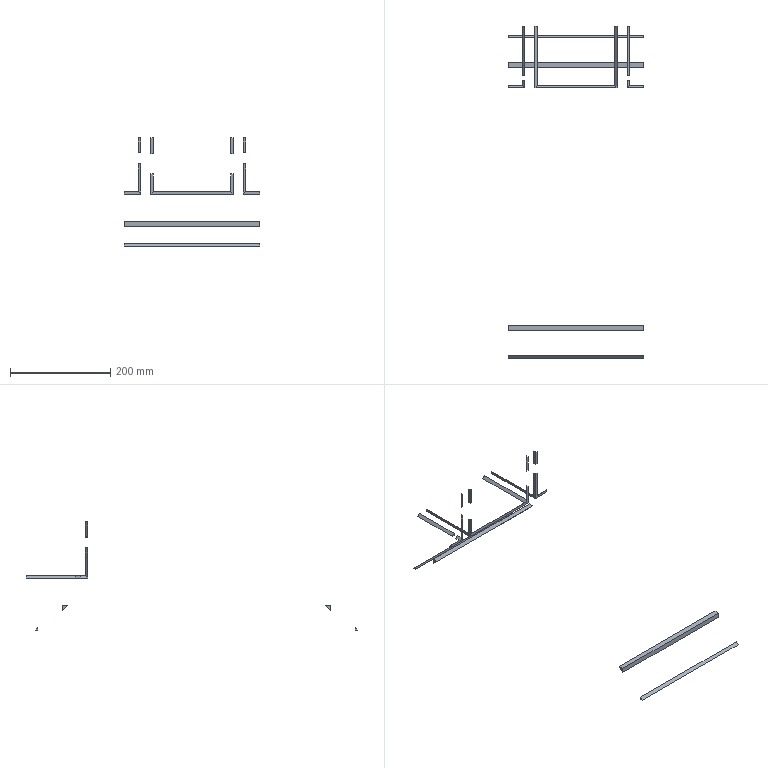Part | STEP file | MAT BAN GIUA_Welds | 13 solids | 81 faces | box 270 x 661.6 x 216 mm | volume 46200 mm3 | plane 81